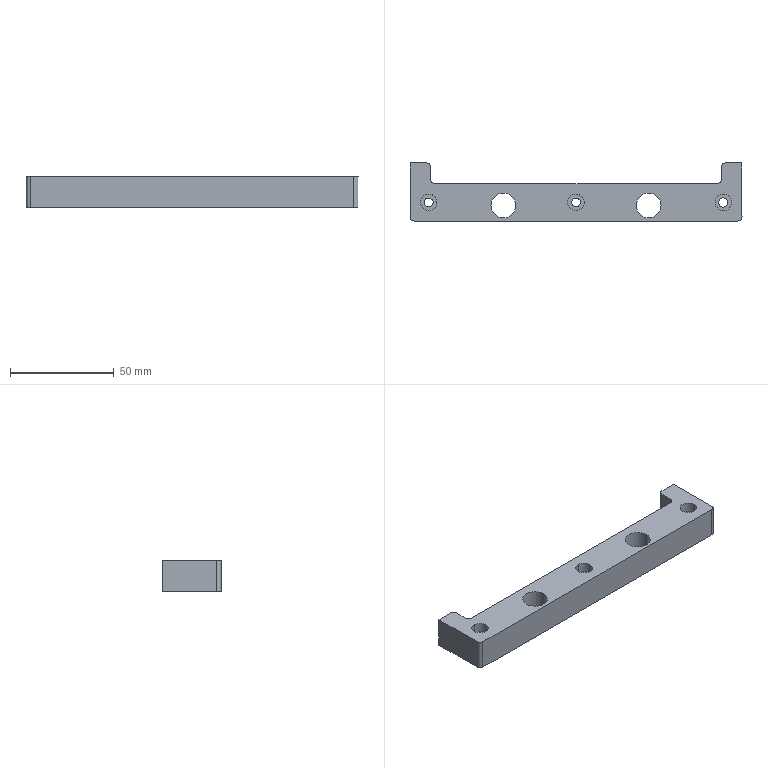Part | SolidWorks | features BaseBody 1, HoleWzd 1, MoveFace 1 | 1 solid | 39 faces | box 160 x 28 x 15 mm | volume 41591 mm3 | cylinder 26 | plane 13 | commonest cylinder face diameters 8 x8 4 x6 4.2 x6 12 x4 4.5 x2
STEP:
#1=CARTESIAN_POINT('',(-666.13,617.297,352.482));
#2=VERTEX_POINT('',#1);
#3=CARTESIAN_POINT('',(-658.13,617.297,352.482));
#4=VERTEX_POINT('',#3);
#5=CARTESIAN_POINT('',(-662.13,617.297,352.482));
#6=DIRECTION('',(0.,0.,1.));
#7=DIRECTION('',(1.,0.,0.));
#8=AXIS2_PLACEMENT_3D('',#5,#6,#7);
#9=CIRCLE('',#8,4.);
#10=EDGE_CURVE('',#2,#4,#9,.T.);
#11=ORIENTED_EDGE('',*,*,#10,.F.);
#12=CARTESIAN_POINT('',(-666.13,617.297,357.482));
#13=VERTEX_POINT('',#12);
#14=CARTESIAN_POINT('',(-666.13,617.297,357.482));
#15=DIRECTION('',(0.,0.,1.));
#16=VECTOR('',#15,1000.);
#17=LINE('',#14,#16);
#18=EDGE_CURVE('',#2,#13,#17,.T.);
#19=ORIENTED_EDGE('',*,*,#18,.T.);
#20=CARTESIAN_POINT('',(-658.13,617.297,357.482));
#21=VERTEX_POINT('',#20);
#22=CARTESIAN_POINT('',(-662.13,617.297,357.482));
#23=DIRECTION('',(0.,0.,1.));
#24=DIRECTION('',(1.,0.,0.));
#25=AXIS2_PLACEMENT_3D('',#22,#23,#24);
#26=CIRCLE('',#25,4.);
#27=EDGE_CURVE('',#13,#21,#26,.T.);
#28=ORIENTED_EDGE('',*,*,#27,.T.);
#29=CARTESIAN_POINT('',(-658.13,617.297,357.482));
#30=DIRECTION('',(0.,0.,1.));
#31=VECTOR('',#30,1000.);
#32=LINE('',#29,#31);
#33=EDGE_CURVE('',#4,#21,#32,.T.);
#34=ORIENTED_EDGE('',*,*,#33,.F.);
#35=EDGE_LOOP('',(#11,#19,#28,#34));
#36=FACE_OUTER_BOUND('',#35,.T.);
#37=CARTESIAN_POINT('',(-662.13,617.297,357.482));
#38=DIRECTION('',(0.,0.,1.));
#39=DIRECTION('',(1.,0.,0.));
#40=AXIS2_PLACEMENT_3D('',#37,#38,#39);
#41=CYLINDRICAL_SURFACE('',#40,4.);
#42=ADVANCED_FACE('',(#36),#41,.F.);
#43=CARTESIAN_POINT('',(-664.38,617.297,342.482));
#44=VERTEX_POINT('',#43);
#45=CARTESIAN_POINT('',(-659.88,617.297,342.482));
#46=VERTEX_POINT('',#45);
#47=CARTESIAN_POINT('',(-662.13,617.297,342.482));
#48=DIRECTION('',(0.,0.,1.));
#49=DIRECTION('',(1.,0.,0.));
#50=AXIS2_PLACEMENT_3D('',#47,#48,#49);
#51=CIRCLE('',#50,2.25);
#52=EDGE_CURVE('',#44,#46,#51,.T.);
#53=ORIENTED_EDGE('',*,*,#52,.F.);
#54=CARTESIAN_POINT('',(-664.38,617.297,352.482));
#55=VERTEX_POINT('',#54);
#56=CARTESIAN_POINT('',(-664.38,617.297,357.482));
#57=DIRECTION('',(0.,0.,1.));
#58=VECTOR('',#57,1000.);
#59=LINE('',#56,#58);
#60=EDGE_CURVE('',#44,#55,#59,.T.);
#61=ORIENTED_EDGE('',*,*,#60,.T.);
#62=CARTESIAN_POINT('',(-659.88,617.297,352.482));
#63=VERTEX_POINT('',#62);
#64=CARTESIAN_POINT('',(-662.13,617.297,352.482));
#65=DIRECTION('',(0.,0.,1.));
#66=DIRECTION('',(1.,0.,0.));
#67=AXIS2_PLACEMENT_3D('',#64,#65,#66);
#68=CIRCLE('',#67,2.25);
#69=EDGE_CURVE('',#55,#63,#68,.T.);
#70=ORIENTED_EDGE('',*,*,#69,.T.);
#71=CARTESIAN_POINT('',(-659.88,617.297,357.482));
#72=DIRECTION('',(0.,0.,1.));
#73=VECTOR('',#72,1000.);
#74=LINE('',#71,#73);
#75=EDGE_CURVE('',#46,#63,#74,.T.);
#76=ORIENTED_EDGE('',*,*,#75,.F.);
#77=EDGE_LOOP('',(#53,#61,#70,#76));
#78=FACE_OUTER_BOUND('',#77,.T.);
#79=CARTESIAN_POINT('',(-662.13,617.297,357.482));
#80=DIRECTION('',(0.,0.,1.));
#81=DIRECTION('',(1.,0.,0.));
#82=AXIS2_PLACEMENT_3D('',#79,#80,#81);
#83=CYLINDRICAL_SURFACE('',#82,2.25);
#84=ADVANCED_FACE('',(#78),#83,.F.);
#85=CARTESIAN_POINT('',(-733.13,615.197,342.482));
#86=VERTEX_POINT('',#85);
#87=CARTESIAN_POINT('',(-735.23,617.297,342.482));
#88=VERTEX_POINT('',#87);
#89=CARTESIAN_POINT('',(-733.13,617.297,342.482));
#90=DIRECTION('',(0.,0.,-1.));
#91=DIRECTION('',(-1.,-0.000001544,0.));
#92=AXIS2_PLACEMENT_3D('',#89,#90,#91);
#93=CIRCLE('',#92,2.1);
#94=EDGE_CURVE('',#86,#88,#93,.T.);
#95=ORIENTED_EDGE('',*,*,#94,.T.);
#96=CARTESIAN_POINT('',(-735.23,617.297,352.482));
#97=VERTEX_POINT('',#96);
#98=CARTESIAN_POINT('',(-735.23,617.297,357.482));
#99=DIRECTION('',(0.,0.,1.));
#100=VECTOR('',#99,1000.);
#101=LINE('',#98,#100);
#102=EDGE_CURVE('',#88,#97,#101,.T.);
#103=ORIENTED_EDGE('',*,*,#102,.T.);
#104=CARTESIAN_POINT('',(-733.13,615.197,352.482));
#105=VERTEX_POINT('',#104);
#106=CARTESIAN_POINT('',(-733.13,617.297,352.482));
#107=DIRECTION('',(0.,0.,1.));
#108=DIRECTION('',(-1.,-0.000001544,0.));
#109=AXIS2_PLACEMENT_3D('',#106,#107,#108);
#110=CIRCLE('',#109,2.1);
#111=EDGE_CURVE('',#97,#105,#110,.T.);
#112=ORIENTED_EDGE('',*,*,#111,.T.);
#113=CARTESIAN_POINT('',(-733.13,615.197,352.482));
#114=DIRECTION('',(0.,0.,-1.));
#115=VECTOR('',#114,1000.);
#116=LINE('',#113,#115);
#117=EDGE_CURVE('',#105,#86,#116,.T.);
#118=ORIENTED_EDGE('',*,*,#117,.T.);
#119=EDGE_LOOP('',(#95,#103,#112,#118));
#120=FACE_OUTER_BOUND('',#119,.T.);
#121=CARTESIAN_POINT('',(-733.13,617.297,357.482));
#122=DIRECTION('',(0.,0.,1.));
#123=DIRECTION('',(-1.,-0.000001544,0.));
#124=AXIS2_PLACEMENT_3D('',#121,#122,#123);
#125=CYLINDRICAL_SURFACE('',#124,2.1);
#126=ADVANCED_FACE('',(#120),#125,.F.);
#127=CARTESIAN_POINT('',(-733.13,613.297,352.482));
#128=VERTEX_POINT('',#127);
#129=CARTESIAN_POINT('',(-737.13,617.297,352.482));
#130=VERTEX_POINT('',#129);
#131=CARTESIAN_POINT('',(-733.13,617.297,352.482));
#132=DIRECTION('',(0.,0.,-1.));
#133=DIRECTION('',(-1.,-0.000001544,0.));
#134=AXIS2_PLACEMENT_3D('',#131,#132,#133);
#135=CIRCLE('',#134,4.);
#136=EDGE_CURVE('',#128,#130,#135,.T.);
#137=ORIENTED_EDGE('',*,*,#136,.T.);
#138=CARTESIAN_POINT('',(-737.13,617.297,357.482));
#139=VERTEX_POINT('',#138);
#140=CARTESIAN_POINT('',(-737.13,617.297,357.482));
#141=DIRECTION('',(0.,0.,1.));
#142=VECTOR('',#141,1000.);
#143=LINE('',#140,#142);
#144=EDGE_CURVE('',#130,#139,#143,.T.);
#145=ORIENTED_EDGE('',*,*,#144,.T.);
#146=CARTESIAN_POINT('',(-733.13,613.297,357.482));
#147=VERTEX_POINT('',#146);
#148=CARTESIAN_POINT('',(-733.13,617.297,357.482));
#149=DIRECTION('',(0.,0.,1.));
#150=DIRECTION('',(-1.,-0.000001544,0.));
#151=AXIS2_PLACEMENT_3D('',#148,#149,#150);
#152=CIRCLE('',#151,4.);
#153=EDGE_CURVE('',#139,#147,#152,.T.);
#154=ORIENTED_EDGE('',*,*,#153,.T.);
#155=CARTESIAN_POINT('',(-733.13,613.297,357.482));
#156=DIRECTION('',(0.,0.,-1.));
#157=VECTOR('',#156,1000.);
#158=LINE('',#155,#157);
#159=EDGE_CURVE('',#147,#128,#158,.T.);
#160=ORIENTED_EDGE('',*,*,#159,.T.);
#161=EDGE_LOOP('',(#137,#145,#154,#160));
#162=FACE_OUTER_BOUND('',#161,.T.);
#163=CARTESIAN_POINT('',(-733.13,617.297,357.482));
#164=DIRECTION('',(0.,0.,1.));
#165=DIRECTION('',(-1.,-0.000001544,0.));
#166=AXIS2_PLACEMENT_3D('',#163,#164,#165);
#167=CYLINDRICAL_SURFACE('',#166,4.);
#168=ADVANCED_FACE('',(#162),#167,.F.);
#169=CARTESIAN_POINT('',(-804.13,615.197,342.482));
#170=VERTEX_POINT('',#169);
#171=CARTESIAN_POINT('',(-806.23,617.297,342.482));
#172=VERTEX_POINT('',#171);
#173=CARTESIAN_POINT('',(-804.13,617.297,342.482));
#174=DIRECTION('',(0.,0.,-1.));
#175=DIRECTION('',(-1.,-0.000001544,0.));
#176=AXIS2_PLACEMENT_3D('',#173,#174,#175);
#177=CIRCLE('',#176,2.1);
#178=EDGE_CURVE('',#170,#172,#177,.T.);
#179=ORIENTED_EDGE('',*,*,#178,.T.);
#180=CARTESIAN_POINT('',(-806.23,617.297,352.482));
#181=VERTEX_POINT('',#180);
#182=CARTESIAN_POINT('',(-806.23,617.297,357.482));
#183=DIRECTION('',(0.,0.,1.));
#184=VECTOR('',#183,1000.);
#185=LINE('',#182,#184);
#186=EDGE_CURVE('',#172,#181,#185,.T.);
#187=ORIENTED_EDGE('',*,*,#186,.T.);
#188=CARTESIAN_POINT('',(-804.13,615.197,352.482));
#189=VERTEX_POINT('',#188);
#190=CARTESIAN_POINT('',(-804.13,617.297,352.482));
#191=DIRECTION('',(0.,0.,1.));
#192=DIRECTION('',(-1.,-0.000001544,0.));
#193=AXIS2_PLACEMENT_3D('',#190,#191,#192);
#194=CIRCLE('',#193,2.1);
#195=EDGE_CURVE('',#181,#189,#194,.T.);
#196=ORIENTED_EDGE('',*,*,#195,.T.);
#197=CARTESIAN_POINT('',(-804.13,615.197,352.482));
#198=DIRECTION('',(0.,0.,-1.));
#199=VECTOR('',#198,1000.);
#200=LINE('',#197,#199);
#201=EDGE_CURVE('',#189,#170,#200,.T.);
#202=ORIENTED_EDGE('',*,*,#201,.T.);
#203=EDGE_LOOP('',(#179,#187,#196,#202));
#204=FACE_OUTER_BOUND('',#203,.T.);
#205=CARTESIAN_POINT('',(-804.13,617.297,357.482));
#206=DIRECTION('',(0.,0.,1.));
#207=DIRECTION('',(-1.,-0.000001544,0.));
#208=AXIS2_PLACEMENT_3D('',#205,#206,#207);
#209=CYLINDRICAL_SURFACE('',#208,2.1);
#210=ADVANCED_FACE('',(#204),#209,.F.);
#211=CARTESIAN_POINT('',(-804.13,613.297,352.482));
#212=VERTEX_POINT('',#211);
#213=CARTESIAN_POINT('',(-808.13,617.297,352.482));
#214=VERTEX_POINT('',#213);
#215=CARTESIAN_POINT('',(-804.13,617.297,352.482));
#216=DIRECTION('',(0.,0.,-1.));
#217=DIRECTION('',(-1.,-0.000001544,0.));
#218=AXIS2_PLACEMENT_3D('',#215,#216,#217);
#219=CIRCLE('',#218,4.);
#220=EDGE_CURVE('',#212,#214,#219,.T.);
#221=ORIENTED_EDGE('',*,*,#220,.T.);
#222=CARTESIAN_POINT('',(-808.13,617.297,357.482));
#223=VERTEX_POINT('',#222);
#224=CARTESIAN_POINT('',(-808.13,617.297,357.482));
#225=DIRECTION('',(0.,0.,1.));
#226=VECTOR('',#225,1000.);
#227=LINE('',#224,#226);
#228=EDGE_CURVE('',#214,#223,#227,.T.);
#229=ORIENTED_EDGE('',*,*,#228,.T.);
#230=CARTESIAN_POINT('',(-804.13,613.297,357.482));
#231=VERTEX_POINT('',#230);
#232=CARTESIAN_POINT('',(-804.13,617.297,357.482));
#233=DIRECTION('',(0.,0.,1.));
#234=DIRECTION('',(-1.,-0.000001544,0.));
#235=AXIS2_PLACEMENT_3D('',#232,#233,#234);
#236=CIRCLE('',#235,4.);
#237=EDGE_CURVE('',#223,#231,#236,.T.);
#238=ORIENTED_EDGE('',*,*,#237,.T.);
#239=CARTESIAN_POINT('',(-804.13,613.297,357.482));
#240=DIRECTION('',(0.,0.,-1.));
#241=VECTOR('',#240,1000.);
#242=LINE('',#239,#241);
#243=EDGE_CURVE('',#231,#212,#242,.T.);
#244=ORIENTED_EDGE('',*,*,#243,.T.);
#245=EDGE_LOOP('',(#221,#229,#238,#244));
#246=FACE_OUTER_BOUND('',#245,.T.);
#247=CARTESIAN_POINT('',(-804.13,617.297,357.482));
#248=DIRECTION('',(0.,0.,1.));
#249=DIRECTION('',(-1.,-0.000001544,0.));
#250=AXIS2_PLACEMENT_3D('',#247,#248,#249);
#251=CYLINDRICAL_SURFACE('',#250,4.);
#252=ADVANCED_FACE('',(#246),#251,.F.);
#253=CARTESIAN_POINT('',(-774.13,615.797,342.482));
#254=VERTEX_POINT('',#253);
#255=CARTESIAN_POINT('',(-762.13,615.797,342.482));
#256=VERTEX_POINT('',#255);
#257=CARTESIAN_POINT('',(-768.13,615.797,342.482));
#258=DIRECTION('',(0.,0.,-1.));
#259=DIRECTION('',(-1.,-0.000001544,0.));
#260=AXIS2_PLACEMENT_3D('',#257,#258,#259);
#261=CIRCLE('',#260,6.);
#262=EDGE_CURVE('',#254,#256,#261,.T.);
#263=ORIENTED_EDGE('',*,*,#262,.F.);
#264=CARTESIAN_POINT('',(-768.13,615.797,342.482));
#265=DIRECTION('',(0.,0.,-1.));
#266=DIRECTION('',(1.,0.000001544,0.));
#267=AXIS2_PLACEMENT_3D('',#264,#265,#266);
#268=CIRCLE('',#267,6.);
#269=EDGE_CURVE('',#256,#254,#268,.T.);
#270=ORIENTED_EDGE('',*,*,#269,.F.);
#271=EDGE_LOOP('',(#263,#270));
#272=FACE_BOUND('',#271,.T.);
#273=CARTESIAN_POINT('',(-704.13,615.797,342.482));
#274=VERTEX_POINT('',#273);
#275=CARTESIAN_POINT('',(-692.13,615.797,342.482));
#276=VERTEX_POINT('',#275);
#277=CARTESIAN_POINT('',(-698.13,615.797,342.482));
#278=DIRECTION('',(0.,0.,-1.));
#279=DIRECTION('',(-1.,-0.000001544,0.));
#280=AXIS2_PLACEMENT_3D('',#277,#278,#279);
#281=CIRCLE('',#280,6.);
#282=EDGE_CURVE('',#274,#276,#281,.T.);
#283=ORIENTED_EDGE('',*,*,#282,.F.);
#284=CARTESIAN_POINT('',(-698.13,615.797,342.482));
#285=DIRECTION('',(0.,0.,-1.));
#286=DIRECTION('',(1.,0.000001544,0.));
#287=AXIS2_PLACEMENT_3D('',#284,#285,#286);
#288=CIRCLE('',#287,6.);
#289=EDGE_CURVE('',#276,#274,#288,.T.);
#290=ORIENTED_EDGE('',*,*,#289,.F.);
#291=EDGE_LOOP('',(#283,#290));
#292=FACE_BOUND('',#291,.T.);
#293=ORIENTED_EDGE('',*,*,#94,.F.);
#294=CARTESIAN_POINT('',(-733.13,619.397,342.482));
#295=VERTEX_POINT('',#294);
#296=CARTESIAN_POINT('',(-733.13,617.297,342.482));
#297=DIRECTION('',(0.,0.,-1.));
#298=DIRECTION('',(-0.000001544,1.,0.));
#299=AXIS2_PLACEMENT_3D('',#296,#297,#298);
#300=CIRCLE('',#299,2.1);
#301=EDGE_CURVE('',#295,#86,#300,.T.);
#302=ORIENTED_EDGE('',*,*,#301,.F.);
#303=CARTESIAN_POINT('',(-733.13,617.297,342.482));
#304=DIRECTION('',(0.,0.,-1.));
#305=DIRECTION('',(-1.,-0.000001544,0.));
#306=AXIS2_PLACEMENT_3D('',#303,#304,#305);
#307=CIRCLE('',#306,2.1);
#308=EDGE_CURVE('',#88,#295,#307,.T.);
#309=ORIENTED_EDGE('',*,*,#308,.F.);
#310=EDGE_LOOP('',(#293,#302,#309));
#311=FACE_BOUND('',#310,.T.);
#312=ORIENTED_EDGE('',*,*,#178,.F.);
#313=CARTESIAN_POINT('',(-804.13,619.397,342.482));
#314=VERTEX_POINT('',#313);
#315=CARTESIAN_POINT('',(-804.13,617.297,342.482));
#316=DIRECTION('',(0.,0.,-1.));
#317=DIRECTION('',(-0.000001544,1.,0.));
#318=AXIS2_PLACEMENT_3D('',#315,#316,#317);
#319=CIRCLE('',#318,2.1);
#320=EDGE_CURVE('',#314,#170,#319,.T.);
#321=ORIENTED_EDGE('',*,*,#320,.F.);
#322=CARTESIAN_POINT('',(-804.13,617.297,342.482));
#323=DIRECTION('',(0.,0.,-1.));
#324=DIRECTION('',(-1.,-0.000001544,0.));
#325=AXIS2_PLACEMENT_3D('',#322,#323,#324);
#326=CIRCLE('',#325,2.1);
#327=EDGE_CURVE('',#172,#314,#326,.T.);
#328=ORIENTED_EDGE('',*,*,#327,.F.);
#329=EDGE_LOOP('',(#312,#321,#328));
#330=FACE_BOUND('',#329,.T.);
#331=CARTESIAN_POINT('',(-653.13,636.297,342.482));
#332=VERTEX_POINT('',#331);
#333=CARTESIAN_POINT('',(-661.13,636.297,342.482));
#334=VERTEX_POINT('',#333);
#335=CARTESIAN_POINT('',(-653.13,636.297,342.482));
#336=DIRECTION('',(-1.,-0.000001544,0.));
#337=VECTOR('',#336,1000.);
#338=LINE('',#335,#337);
#339=EDGE_CURVE('',#332,#334,#338,.T.);
#340=ORIENTED_EDGE('',*,*,#339,.F.);
#341=CARTESIAN_POINT('',(-653.13,610.297,342.482));
#342=VERTEX_POINT('',#341);
#343=CARTESIAN_POINT('',(-653.13,610.297,342.482));
#344=DIRECTION('',(-0.000001544,1.,0.));
#345=VECTOR('',#344,1000.);
#346=LINE('',#343,#345);
#347=EDGE_CURVE('',#342,#332,#346,.T.);
#348=ORIENTED_EDGE('',*,*,#347,.F.);
#349=CARTESIAN_POINT('',(-655.13,608.297,342.482));
#350=VERTEX_POINT('',#349);
#351=CARTESIAN_POINT('',(-655.13,610.297,342.482));
#352=DIRECTION('',(0.,0.,1.));
#353=DIRECTION('',(0.000001545,-1.,0.));
#354=AXIS2_PLACEMENT_3D('',#351,#352,#353);
#355=CIRCLE('',#354,2.);
#356=EDGE_CURVE('',#350,#342,#355,.T.);
#357=ORIENTED_EDGE('',*,*,#356,.F.);
#358=CARTESIAN_POINT('',(-811.13,608.297,342.482));
#359=VERTEX_POINT('',#358);
#360=CARTESIAN_POINT('',(-811.13,608.297,342.482));
#361=DIRECTION('',(1.,0.000001544,0.));
#362=VECTOR('',#361,1000.);
#363=LINE('',#360,#362);
#364=EDGE_CURVE('',#359,#350,#363,.T.);
#365=ORIENTED_EDGE('',*,*,#364,.F.);
#366=CARTESIAN_POINT('',(-813.13,610.297,342.482));
#367=VERTEX_POINT('',#366);
#368=CARTESIAN_POINT('',(-811.13,610.297,342.482));
#369=DIRECTION('',(0.,0.,1.));
#370=DIRECTION('',(-1.,-0.000001545,0.));
#371=AXIS2_PLACEMENT_3D('',#368,#369,#370);
#372=CIRCLE('',#371,2.);
#373=EDGE_CURVE('',#367,#359,#372,.T.);
#374=ORIENTED_EDGE('',*,*,#373,.F.);
#375=CARTESIAN_POINT('',(-813.13,636.297,342.482));
#376=VERTEX_POINT('',#375);
#377=CARTESIAN_POINT('',(-813.13,636.297,342.482));
#378=DIRECTION('',(0.000001544,-1.,0.));
#379=VECTOR('',#378,1000.);
#380=LINE('',#377,#379);
#381=EDGE_CURVE('',#376,#367,#380,.T.);
#382=ORIENTED_EDGE('',*,*,#381,.F.);
#383=CARTESIAN_POINT('',(-805.13,636.297,342.482));
#384=VERTEX_POINT('',#383);
#385=CARTESIAN_POINT('',(-805.13,636.297,342.482));
#386=DIRECTION('',(-1.,-0.000001544,0.));
#387=VECTOR('',#386,1000.);
#388=LINE('',#385,#387);
#389=EDGE_CURVE('',#384,#376,#388,.T.);
#390=ORIENTED_EDGE('',*,*,#389,.F.);
#391=CARTESIAN_POINT('',(-803.13,634.297,342.482));
#392=VERTEX_POINT('',#391);
#393=CARTESIAN_POINT('',(-805.13,634.297,342.482));
#394=DIRECTION('',(0.,0.,1.));
#395=DIRECTION('',(1.,0.000001543,0.));
#396=AXIS2_PLACEMENT_3D('',#393,#394,#395);
#397=CIRCLE('',#396,2.);
#398=EDGE_CURVE('',#392,#384,#397,.T.);
#399=ORIENTED_EDGE('',*,*,#398,.F.);
#400=CARTESIAN_POINT('',(-803.13,628.297,342.482));
#401=VERTEX_POINT('',#400);
#402=CARTESIAN_POINT('',(-803.13,634.297,342.482));
#403=DIRECTION('',(0.000001544,-1.,0.));
#404=VECTOR('',#403,1000.);
#405=LINE('',#402,#404);
#406=EDGE_CURVE('',#392,#401,#405,.T.);
#407=ORIENTED_EDGE('',*,*,#406,.T.);
#408=CARTESIAN_POINT('',(-801.13,626.297,342.482));
#409=VERTEX_POINT('',#408);
#410=CARTESIAN_POINT('',(-801.13,628.297,342.482));
#411=DIRECTION('',(0.,0.,-1.));
#412=DIRECTION('',(0.000001545,-1.,0.));
#413=AXIS2_PLACEMENT_3D('',#410,#411,#412);
#414=CIRCLE('',#413,2.);
#415=EDGE_CURVE('',#409,#401,#414,.T.);
#416=ORIENTED_EDGE('',*,*,#415,.F.);
#417=CARTESIAN_POINT('',(-665.13,626.297,342.482));
#418=VERTEX_POINT('',#417);
#419=CARTESIAN_POINT('',(-801.13,626.297,342.482));
#420=DIRECTION('',(1.,0.000001544,0.));
#421=VECTOR('',#420,1000.);
#422=LINE('',#419,#421);
#423=EDGE_CURVE('',#409,#418,#422,.T.);
#424=ORIENTED_EDGE('',*,*,#423,.T.);
#425=CARTESIAN_POINT('',(-663.13,628.297,342.482));
#426=VERTEX_POINT('',#425);
#427=CARTESIAN_POINT('',(-665.13,628.297,342.482));
#428=DIRECTION('',(0.,0.,-1.));
#429=DIRECTION('',(1.,0.000001545,0.));
#430=AXIS2_PLACEMENT_3D('',#427,#428,#429);
#431=CIRCLE('',#430,2.);
#432=EDGE_CURVE('',#426,#418,#431,.T.);
#433=ORIENTED_EDGE('',*,*,#432,.F.);
#434=CARTESIAN_POINT('',(-663.13,634.297,342.482));
#435=VERTEX_POINT('',#434);
#436=CARTESIAN_POINT('',(-663.13,634.297,342.482));
#437=DIRECTION('',(0.000001544,-1.,0.));
#438=VECTOR('',#437,1000.);
#439=LINE('',#436,#438);
#440=EDGE_CURVE('',#435,#426,#439,.T.);
#441=ORIENTED_EDGE('',*,*,#440,.F.);
#442=CARTESIAN_POINT('',(-661.13,634.297,342.482));
#443=DIRECTION('',(0.,0.,1.));
#444=DIRECTION('',(-0.000001544,1.,0.));
#445=AXIS2_PLACEMENT_3D('',#442,#443,#444);
#446=CIRCLE('',#445,2.);
#447=EDGE_CURVE('',#334,#435,#446,.T.);
#448=ORIENTED_EDGE('',*,*,#447,.F.);
#449=EDGE_LOOP('',(#340,#348,#357,#365,#374,#382,#390,#399,#407,#416,#424,#433,#441,#448));
#450=FACE_OUTER_BOUND('',#449,.T.);
#451=CARTESIAN_POINT('',(-662.13,617.297,342.482));
#452=DIRECTION('',(0.,0.,1.));
#453=DIRECTION('',(1.,0.,0.));
#454=AXIS2_PLACEMENT_3D('',#451,#452,#453);
#455=CIRCLE('',#454,2.25);
#456=EDGE_CURVE('',#46,#44,#455,.T.);
#457=ORIENTED_EDGE('',*,*,#456,.T.);
#458=ORIENTED_EDGE('',*,*,#52,.T.);
#459=EDGE_LOOP('',(#457,#458));
#460=FACE_BOUND('',#459,.T.);
#461=CARTESIAN_POINT('',(-653.13,608.297,342.482));
#462=DIRECTION('',(0.,0.,-1.));
#463=DIRECTION('',(0.000001544,-1.,0.));
#464=AXIS2_PLACEMENT_3D('',#461,#462,#463);
#465=PLANE('',#464);
#466=ADVANCED_FACE('',(#272,#292,#311,#330,#450,#460),#465,.T.);
#467=CARTESIAN_POINT('',(-803.13,634.297,357.482));
#468=VERTEX_POINT('',#467);
#469=CARTESIAN_POINT('',(-803.13,634.297,342.482));
#470=DIRECTION('',(0.,0.,1.));
#471=VECTOR('',#470,1000.);
#472=LINE('',#469,#471);
#473=EDGE_CURVE('',#392,#468,#472,.T.);
#474=ORIENTED_EDGE('',*,*,#473,.T.);
#475=CARTESIAN_POINT('',(-803.13,628.297,357.482));
#476=VERTEX_POINT('',#475);
#477=CARTESIAN_POINT('',(-803.13,628.297,357.482));
#478=DIRECTION('',(-0.000001544,1.,0.));
#479=VECTOR('',#478,1000.);
#480=LINE('',#477,#479);
#481=EDGE_CURVE('',#476,#468,#480,.T.);
#482=ORIENTED_EDGE('',*,*,#481,.F.);
#483=CARTESIAN_POINT('',(-803.13,628.297,357.482));
#484=DIRECTION('',(0.,0.,-1.));
#485=VECTOR('',#484,1000.);
#486=LINE('',#483,#485);
#487=EDGE_CURVE('',#476,#401,#486,.T.);
#488=ORIENTED_EDGE('',*,*,#487,.T.);
#489=ORIENTED_EDGE('',*,*,#406,.F.);
#490=EDGE_LOOP('',(#474,#482,#488,#489));
#491=FACE_OUTER_BOUND('',#490,.T.);
#492=CARTESIAN_POINT('',(-803.13,626.297,357.482));
#493=DIRECTION('',(1.,0.000001544,0.));
#494=DIRECTION('',(0.000001544,-1.,0.));
#495=AXIS2_PLACEMENT_3D('',#492,#493,#494);
#496=PLANE('',#495);
#497=ADVANCED_FACE('',(#491),#496,.T.);
#498=CARTESIAN_POINT('',(-663.13,634.297,357.482));
#499=VERTEX_POINT('',#498);
#500=CARTESIAN_POINT('',(-661.13,636.297,357.482));
#501=VERTEX_POINT('',#500);
#502=CARTESIAN_POINT('',(-661.13,634.297,357.482));
#503=DIRECTION('',(0.,0.,-1.));
#504=DIRECTION('',(-1.,-0.000001544,0.));
#505=AXIS2_PLACEMENT_3D('',#502,#503,#504);
#506=CIRCLE('',#505,2.);
#507=EDGE_CURVE('',#499,#501,#506,.T.);
#508=ORIENTED_EDGE('',*,*,#507,.T.);
#509=CARTESIAN_POINT('',(-661.13,636.297,342.482));
#510=DIRECTION('',(0.,0.,1.));
#511=VECTOR('',#510,1000.);
#512=LINE('',#509,#511);
#513=EDGE_CURVE('',#334,#501,#512,.T.);
#514=ORIENTED_EDGE('',*,*,#513,.F.);
#515=ORIENTED_EDGE('',*,*,#447,.T.);
#516=CARTESIAN_POINT('',(-663.13,634.297,357.482));
#517=DIRECTION('',(0.,0.,-1.));
#518=VECTOR('',#517,1000.);
#519=LINE('',#516,#518);
#520=EDGE_CURVE('',#499,#435,#519,.T.);
#521=ORIENTED_EDGE('',*,*,#520,.F.);
#522=EDGE_LOOP('',(#508,#514,#515,#521));
#523=FACE_OUTER_BOUND('',#522,.T.);
#524=CARTESIAN_POINT('',(-661.13,634.297,494.293));
#525=DIRECTION('',(0.,0.,-1.));
#526=DIRECTION('',(1.,0.000001544,0.));
#527=AXIS2_PLACEMENT_3D('',#524,#525,#526);
#528=CYLINDRICAL_SURFACE('',#527,2.);
#529=ADVANCED_FACE('',(#523),#528,.T.);
#530=ORIENTED_EDGE('',*,*,#520,.T.);
#531=ORIENTED_EDGE('',*,*,#440,.T.);
#532=CARTESIAN_POINT('',(-663.13,628.297,357.482));
#533=VERTEX_POINT('',#532);
#534=CARTESIAN_POINT('',(-663.13,628.297,342.482));
#535=DIRECTION('',(0.,0.,1.));
#536=VECTOR('',#535,1000.);
#537=LINE('',#534,#536);
#538=EDGE_CURVE('',#426,#533,#537,.T.);
#539=ORIENTED_EDGE('',*,*,#538,.T.);
#540=CARTESIAN_POINT('',(-663.13,634.297,357.482));
#541=DIRECTION('',(0.000001544,-1.,0.));
#542=VECTOR('',#541,1000.);
#543=LINE('',#540,#542);
#544=EDGE_CURVE('',#499,#533,#543,.T.);
#545=ORIENTED_EDGE('',*,*,#544,.F.);
#546=EDGE_LOOP('',(#530,#531,#539,#545));
#547=FACE_OUTER_BOUND('',#546,.T.);
#548=CARTESIAN_POINT('',(-663.13,636.297,357.482));
#549=DIRECTION('',(-1.,-0.000001544,0.));
#550=DIRECTION('',(-0.000001544,1.,0.));
#551=AXIS2_PLACEMENT_3D('',#548,#549,#550);
#552=PLANE('',#551);
#553=ADVANCED_FACE('',(#547),#552,.T.);
#554=CARTESIAN_POINT('',(-662.13,617.297,357.482));
#555=DIRECTION('',(0.,0.,1.));
#556=DIRECTION('',(1.,0.,0.));
#557=AXIS2_PLACEMENT_3D('',#554,#555,#556);
#558=CIRCLE('',#557,4.);
#559=EDGE_CURVE('',#21,#13,#558,.T.);
#560=ORIENTED_EDGE('',*,*,#559,.F.);
#561=ORIENTED_EDGE('',*,*,#27,.F.);
#562=EDGE_LOOP('',(#560,#561));
#563=FACE_BOUND('',#562,.T.);
#564=ORIENTED_EDGE('',*,*,#481,.T.);
#565=CARTESIAN_POINT('',(-805.13,636.297,357.482));
#566=VERTEX_POINT('',#565);
#567=CARTESIAN_POINT('',(-805.13,634.297,357.482));
#568=DIRECTION('',(0.,0.,-1.));
#569=DIRECTION('',(-0.000001544,1.,0.));
#570=AXIS2_PLACEMENT_3D('',#567,#568,#569);
#571=CIRCLE('',#570,2.);
#572=EDGE_CURVE('',#566,#468,#571,.T.);
#573=ORIENTED_EDGE('',*,*,#572,.F.);
#574=CARTESIAN_POINT('',(-813.13,636.297,357.482));
#575=VERTEX_POINT('',#574);
#576=CARTESIAN_POINT('',(-813.13,636.297,357.482));
#577=DIRECTION('',(1.,0.000001544,0.));
#578=VECTOR('',#577,1000.);
#579=LINE('',#576,#578);
#580=EDGE_CURVE('',#575,#566,#579,.T.);
#581=ORIENTED_EDGE('',*,*,#580,.F.);
#582=CARTESIAN_POINT('',(-813.13,610.297,357.482));
#583=VERTEX_POINT('',#582);
#584=CARTESIAN_POINT('',(-813.13,610.297,357.482));
#585=DIRECTION('',(-0.000001544,1.,0.));
#586=VECTOR('',#585,1000.);
#587=LINE('',#584,#586);
#588=EDGE_CURVE('',#583,#575,#587,.T.);
#589=ORIENTED_EDGE('',*,*,#588,.F.);
#590=CARTESIAN_POINT('',(-811.13,608.297,357.482));
#591=VERTEX_POINT('',#590);
#592=CARTESIAN_POINT('',(-811.13,610.297,357.482));
#593=DIRECTION('',(0.,0.,-1.));
#594=DIRECTION('',(0.000001545,-1.,0.));
#595=AXIS2_PLACEMENT_3D('',#592,#593,#594);
#596=CIRCLE('',#595,2.);
#597=EDGE_CURVE('',#591,#583,#596,.T.);
#598=ORIENTED_EDGE('',*,*,#597,.F.);
#599=CARTESIAN_POINT('',(-655.13,608.297,357.482));
#600=VERTEX_POINT('',#599);
#601=CARTESIAN_POINT('',(-655.13,608.297,357.482));
#602=DIRECTION('',(-1.,-0.000001544,0.));
#603=VECTOR('',#602,1000.);
#604=LINE('',#601,#603);
#605=EDGE_CURVE('',#600,#591,#604,.T.);
#606=ORIENTED_EDGE('',*,*,#605,.F.);
#607=CARTESIAN_POINT('',(-653.13,610.297,357.482));
#608=VERTEX_POINT('',#607);
#609=CARTESIAN_POINT('',(-655.13,610.297,357.482));
#610=DIRECTION('',(0.,0.,-1.));
#611=DIRECTION('',(1.,0.000001544,0.));
#612=AXIS2_PLACEMENT_3D('',#609,#610,#611);
#613=CIRCLE('',#612,2.);
#614=EDGE_CURVE('',#608,#600,#613,.T.);
#615=ORIENTED_EDGE('',*,*,#614,.F.);
#616=CARTESIAN_POINT('',(-653.13,636.297,357.482));
#617=VERTEX_POINT('',#616);
#618=CARTESIAN_POINT('',(-653.13,636.297,357.482));
#619=DIRECTION('',(0.000001544,-1.,0.));
#620=VECTOR('',#619,1000.);
#621=LINE('',#618,#620);
#622=EDGE_CURVE('',#617,#608,#621,.T.);
#623=ORIENTED_EDGE('',*,*,#622,.F.);
#624=CARTESIAN_POINT('',(-661.13,636.297,357.482));
#625=DIRECTION('',(1.,0.000001544,0.));
#626=VECTOR('',#625,1000.);
#627=LINE('',#624,#626);
#628=EDGE_CURVE('',#501,#617,#627,.T.);
#629=ORIENTED_EDGE('',*,*,#628,.F.);
#630=ORIENTED_EDGE('',*,*,#507,.F.);
#631=ORIENTED_EDGE('',*,*,#544,.T.);
#632=CARTESIAN_POINT('',(-665.13,626.297,357.482));
#633=VERTEX_POINT('',#632);
#634=CARTESIAN_POINT('',(-665.13,628.297,357.482));
#635=DIRECTION('',(0.,0.,1.));
#636=DIRECTION('',(0.000001545,-1.,0.));
#637=AXIS2_PLACEMENT_3D('',#634,#635,#636);
#638=CIRCLE('',#637,2.);
#639=EDGE_CURVE('',#633,#533,#638,.T.);
#640=ORIENTED_EDGE('',*,*,#639,.F.);
#641=CARTESIAN_POINT('',(-801.13,626.297,357.482));
#642=VERTEX_POINT('',#641);
#643=CARTESIAN_POINT('',(-665.13,626.297,357.482));
#644=DIRECTION('',(-1.,-0.000001544,0.));
#645=VECTOR('',#644,1000.);
#646=LINE('',#643,#645);
#647=EDGE_CURVE('',#633,#642,#646,.T.);
#648=ORIENTED_EDGE('',*,*,#647,.T.);
#649=CARTESIAN_POINT('',(-801.13,628.297,357.482));
#650=DIRECTION('',(0.,0.,1.));
#651=DIRECTION('',(-1.,-0.000001544,0.));
#652=AXIS2_PLACEMENT_3D('',#649,#650,#651);
#653=CIRCLE('',#652,2.);
#654=EDGE_CURVE('',#476,#642,#653,.T.);
#655=ORIENTED_EDGE('',*,*,#654,.F.);
#656=EDGE_LOOP('',(#564,#573,#581,#589,#598,#606,#615,#623,#629,#630,#631,#640,#648,#655));
#657=FACE_OUTER_BOUND('',#656,.T.);
#658=CARTESIAN_POINT('',(-804.13,621.297,357.482));
#659=VERTEX_POINT('',#658);
#660=CARTESIAN_POINT('',(-804.13,617.297,357.482));
#661=DIRECTION('',(0.,0.,1.));
#662=DIRECTION('',(-1.,-0.000001544,0.));
#663=AXIS2_PLACEMENT_3D('',#660,#661,#662);
#664=CIRCLE('',#663,4.);
#665=EDGE_CURVE('',#659,#223,#664,.T.);
#666=ORIENTED_EDGE('',*,*,#665,.F.);
#667=CARTESIAN_POINT('',(-804.13,617.297,357.482));
#668=DIRECTION('',(0.,0.,1.));
#669=DIRECTION('',(0.000001544,-1.,0.));
#670=AXIS2_PLACEMENT_3D('',#667,#668,#669);
#671=CIRCLE('',#670,4.);
#672=EDGE_CURVE('',#231,#659,#671,.T.);
#673=ORIENTED_EDGE('',*,*,#672,.F.);
#674=ORIENTED_EDGE('',*,*,#237,.F.);
#675=EDGE_LOOP('',(#666,#673,#674));
#676=FACE_BOUND('',#675,.T.);
#677=CARTESIAN_POINT('',(-733.13,621.297,357.482));
#678=VERTEX_POINT('',#677);
#679=CARTESIAN_POINT('',(-733.13,617.297,357.482));
#680=DIRECTION('',(0.,0.,1.));
#681=DIRECTION('',(-1.,-0.000001544,0.));
#682=AXIS2_PLACEMENT_3D('',#679,#680,#681);
#683=CIRCLE('',#682,4.);
#684=EDGE_CURVE('',#678,#139,#683,.T.);
#685=ORIENTED_EDGE('',*,*,#684,.F.);
#686=CARTESIAN_POINT('',(-733.13,617.297,357.482));
#687=DIRECTION('',(0.,0.,1.));
#688=DIRECTION('',(0.000001544,-1.,0.));
#689=AXIS2_PLACEMENT_3D('',#686,#687,#688);
#690=CIRCLE('',#689,4.);
#691=EDGE_CURVE('',#147,#678,#690,.T.);
#692=ORIENTED_EDGE('',*,*,#691,.F.);
#693=ORIENTED_EDGE('',*,*,#153,.F.);
#694=EDGE_LOOP('',(#685,#692,#693));
#695=FACE_BOUND('',#694,.T.);
#696=CARTESIAN_POINT('',(-692.13,615.797,357.482));
#697=VERTEX_POINT('',#696);
#698=CARTESIAN_POINT('',(-704.13,615.797,357.482));
#699=VERTEX_POINT('',#698);
#700=CARTESIAN_POINT('',(-698.13,615.797,357.482));
#701=DIRECTION('',(0.,0.,1.));
#702=DIRECTION('',(1.,0.000001544,0.));
#703=AXIS2_PLACEMENT_3D('',#700,#701,#702);
#704=CIRCLE('',#703,6.);
#705=EDGE_CURVE('',#697,#699,#704,.T.);
#706=ORIENTED_EDGE('',*,*,#705,.F.);
#707=CARTESIAN_POINT('',(-698.13,615.797,357.482));
#708=DIRECTION('',(0.,0.,1.));
#709=DIRECTION('',(-1.,-0.000001544,0.));
#710=AXIS2_PLACEMENT_3D('',#707,#708,#709);
#711=CIRCLE('',#710,6.);
#712=EDGE_CURVE('',#699,#697,#711,.T.);
#713=ORIENTED_EDGE('',*,*,#712,.F.);
#714=EDGE_LOOP('',(#706,#713));
#715=FACE_BOUND('',#714,.T.);
#716=CARTESIAN_POINT('',(-762.13,615.797,357.482));
#717=VERTEX_POINT('',#716);
#718=CARTESIAN_POINT('',(-774.13,615.797,357.482));
#719=VERTEX_POINT('',#718);
#720=CARTESIAN_POINT('',(-768.13,615.797,357.482));
#721=DIRECTION('',(0.,0.,1.));
#722=DIRECTION('',(1.,0.000001544,0.));
#723=AXIS2_PLACEMENT_3D('',#720,#721,#722);
#724=CIRCLE('',#723,6.);
#725=EDGE_CURVE('',#717,#719,#724,.T.);
#726=ORIENTED_EDGE('',*,*,#725,.F.);
#727=CARTESIAN_POINT('',(-768.13,615.797,357.482));
#728=DIRECTION('',(0.,0.,1.));
#729=DIRECTION('',(-1.,-0.000001544,0.));
#730=AXIS2_PLACEMENT_3D('',#727,#728,#729);
#731=CIRCLE('',#730,6.);
#732=EDGE_CURVE('',#719,#717,#731,.T.);
#733=ORIENTED_EDGE('',*,*,#732,.F.);
#734=EDGE_LOOP('',(#726,#733));
#735=FACE_BOUND('',#734,.T.);
#736=CARTESIAN_POINT('',(-653.13,626.297,357.482));
#737=DIRECTION('',(0.,0.,1.));
#738=DIRECTION('',(-0.000001544,1.,0.));
#739=AXIS2_PLACEMENT_3D('',#736,#737,#738);
#740=PLANE('',#739);
#741=ADVANCED_FACE('',(#563,#657,#676,#695,#715,#735),#740,.T.);
#742=ORIENTED_EDGE('',*,*,#487,.F.);
#743=ORIENTED_EDGE('',*,*,#654,.T.);
#744=CARTESIAN_POINT('',(-801.13,626.297,342.482));
#745=DIRECTION('',(0.,0.,1.));
#746=VECTOR('',#745,1000.);
#747=LINE('',#744,#746);
#748=EDGE_CURVE('',#409,#642,#747,.T.);
#749=ORIENTED_EDGE('',*,*,#748,.F.);
#750=ORIENTED_EDGE('',*,*,#415,.T.);
#751=EDGE_LOOP('',(#742,#743,#749,#750));
#752=FACE_OUTER_BOUND('',#751,.T.);
#753=CARTESIAN_POINT('',(-801.13,628.297,494.293));
#754=DIRECTION('',(0.,0.,-1.));
#755=DIRECTION('',(1.,0.000001544,0.));
#756=AXIS2_PLACEMENT_3D('',#753,#754,#755);
#757=CYLINDRICAL_SURFACE('',#756,2.);
#758=ADVANCED_FACE('',(#752),#757,.F.);
#759=CARTESIAN_POINT('',(-665.13,626.297,357.482));
#760=DIRECTION('',(0.,0.,-1.));
#761=VECTOR('',#760,1000.);
#762=LINE('',#759,#761);
#763=EDGE_CURVE('',#633,#418,#762,.T.);
#764=ORIENTED_EDGE('',*,*,#763,.T.);
#765=ORIENTED_EDGE('',*,*,#423,.F.);
#766=ORIENTED_EDGE('',*,*,#748,.T.);
#767=ORIENTED_EDGE('',*,*,#647,.F.);
#768=EDGE_LOOP('',(#764,#765,#766,#767));
#769=FACE_OUTER_BOUND('',#768,.T.);
#770=CARTESIAN_POINT('',(-653.13,626.297,342.482));
#771=DIRECTION('',(-0.000001544,1.,0.));
#772=DIRECTION('',(0.,0.,-1.));
#773=AXIS2_PLACEMENT_3D('',#770,#771,#772);
#774=PLANE('',#773);
#775=ADVANCED_FACE('',(#769),#774,.T.);
#776=ORIENTED_EDGE('',*,*,#538,.F.);
#777=ORIENTED_EDGE('',*,*,#432,.T.);
#778=ORIENTED_EDGE('',*,*,#763,.F.);
#779=ORIENTED_EDGE('',*,*,#639,.T.);
#780=EDGE_LOOP('',(#776,#777,#778,#779));
#781=FACE_OUTER_BOUND('',#780,.T.);
#782=CARTESIAN_POINT('',(-665.13,628.297,256.572));
#783=DIRECTION('',(0.,0.,1.));
#784=DIRECTION('',(-1.,-0.000001544,0.));
#785=AXIS2_PLACEMENT_3D('',#782,#783,#784);
#786=CYLINDRICAL_SURFACE('',#785,2.);
#787=ADVANCED_FACE('',(#781),#786,.F.);
#788=CARTESIAN_POINT('',(-653.13,636.297,342.482));
#789=DIRECTION('',(0.,0.,1.));
#790=VECTOR('',#789,1000.);
#791=LINE('',#788,#790);
#792=EDGE_CURVE('',#332,#617,#791,.T.);
#793=ORIENTED_EDGE('',*,*,#792,.F.);
#794=ORIENTED_EDGE('',*,*,#339,.T.);
#795=ORIENTED_EDGE('',*,*,#513,.T.);
#796=ORIENTED_EDGE('',*,*,#628,.T.);
#797=EDGE_LOOP('',(#793,#794,#795,#796));
#798=FACE_OUTER_BOUND('',#797,.T.);
#799=CARTESIAN_POINT('',(-653.13,636.297,357.482));
#800=DIRECTION('',(-0.000001544,1.,0.));
#801=DIRECTION('',(1.,0.000001544,0.));
#802=AXIS2_PLACEMENT_3D('',#799,#800,#801);
#803=PLANE('',#802);
#804=ADVANCED_FACE('',(#798),#803,.T.);
#805=ORIENTED_EDGE('',*,*,#792,.T.);
#806=ORIENTED_EDGE('',*,*,#622,.T.);
#807=CARTESIAN_POINT('',(-653.13,610.297,357.482));
#808=DIRECTION('',(0.,0.,-1.));
#809=VECTOR('',#808,1000.);
#810=LINE('',#807,#809);
#811=EDGE_CURVE('',#608,#342,#810,.T.);
#812=ORIENTED_EDGE('',*,*,#811,.T.);
#813=ORIENTED_EDGE('',*,*,#347,.T.);
#814=EDGE_LOOP('',(#805,#806,#812,#813));
#815=FACE_OUTER_BOUND('',#814,.T.);
#816=CARTESIAN_POINT('',(-653.129,0.00034,-0.25));
#817=DIRECTION('',(1.,0.000001544,0.));
#818=DIRECTION('',(0.000001544,-1.,0.));
#819=AXIS2_PLACEMENT_3D('',#816,#817,#818);
#820=PLANE('',#819);
#821=ADVANCED_FACE('',(#815),#820,.T.);
#822=ORIENTED_EDGE('',*,*,#614,.T.);
#823=CARTESIAN_POINT('',(-655.13,608.297,342.482));
#824=DIRECTION('',(0.,0.,1.));
#825=VECTOR('',#824,1000.);
#826=LINE('',#823,#825);
#827=EDGE_CURVE('',#350,#600,#826,.T.);
#828=ORIENTED_EDGE('',*,*,#827,.F.);
#829=ORIENTED_EDGE('',*,*,#356,.T.);
#830=ORIENTED_EDGE('',*,*,#811,.F.);
#831=EDGE_LOOP('',(#822,#828,#829,#830));
#832=FACE_OUTER_BOUND('',#831,.T.);
#833=CARTESIAN_POINT('',(-655.13,610.297,494.293));
#834=DIRECTION('',(0.,0.,-1.));
#835=DIRECTION('',(1.,0.000001544,0.));
#836=AXIS2_PLACEMENT_3D('',#833,#834,#835);
#837=CYLINDRICAL_SURFACE('',#836,2.);
#838=ADVANCED_FACE('',(#832),#837,.T.);
#839=CARTESIAN_POINT('',(-811.13,608.297,357.482));
#840=DIRECTION('',(0.,0.,-1.));
#841=VECTOR('',#840,1000.);
#842=LINE('',#839,#841);
#843=EDGE_CURVE('',#591,#359,#842,.T.);
#844=ORIENTED_EDGE('',*,*,#843,.T.);
#845=ORIENTED_EDGE('',*,*,#364,.T.);
#846=ORIENTED_EDGE('',*,*,#827,.T.);
#847=ORIENTED_EDGE('',*,*,#605,.T.);
#848=EDGE_LOOP('',(#844,#845,#846,#847));
#849=FACE_OUTER_BOUND('',#848,.T.);
#850=CARTESIAN_POINT('',(-653.13,608.297,357.482));
#851=DIRECTION('',(0.000001544,-1.,0.));
#852=DIRECTION('',(0.,0.,1.));
#853=AXIS2_PLACEMENT_3D('',#850,#851,#852);
#854=PLANE('',#853);
#855=ADVANCED_FACE('',(#849),#854,.T.);
#856=ORIENTED_EDGE('',*,*,#373,.T.);
#857=ORIENTED_EDGE('',*,*,#843,.F.);
#858=ORIENTED_EDGE('',*,*,#597,.T.);
#859=CARTESIAN_POINT('',(-813.13,610.297,342.482));
#860=DIRECTION('',(0.,0.,1.));
#861=VECTOR('',#860,1000.);
#862=LINE('',#859,#861);
#863=EDGE_CURVE('',#367,#583,#862,.T.);
#864=ORIENTED_EDGE('',*,*,#863,.F.);
#865=EDGE_LOOP('',(#856,#857,#858,#864));
#866=FACE_OUTER_BOUND('',#865,.T.);
#867=CARTESIAN_POINT('',(-811.13,610.297,256.572));
#868=DIRECTION('',(0.,0.,1.));
#869=DIRECTION('',(-1.,-0.000001544,0.));
#870=AXIS2_PLACEMENT_3D('',#867,#868,#869);
#871=CYLINDRICAL_SURFACE('',#870,2.);
#872=ADVANCED_FACE('',(#866),#871,.T.);
#873=CARTESIAN_POINT('',(-813.13,636.297,342.482));
#874=DIRECTION('',(0.,0.,1.));
#875=VECTOR('',#874,1000.);
#876=LINE('',#873,#875);
#877=EDGE_CURVE('',#376,#575,#876,.T.);
#878=ORIENTED_EDGE('',*,*,#877,.F.);
#879=ORIENTED_EDGE('',*,*,#381,.T.);
#880=ORIENTED_EDGE('',*,*,#863,.T.);
#881=ORIENTED_EDGE('',*,*,#588,.T.);
#882=EDGE_LOOP('',(#878,#879,#880,#881));
#883=FACE_OUTER_BOUND('',#882,.T.);
#884=CARTESIAN_POINT('',(-813.13,738.297,342.482));
#885=DIRECTION('',(1.,0.000001544,0.));
#886=DIRECTION('',(0.000001544,-1.,0.));
#887=AXIS2_PLACEMENT_3D('',#884,#885,#886);
#888=PLANE('',#887);
#889=ADVANCED_FACE('',(#883),#888,.F.);
#890=ORIENTED_EDGE('',*,*,#877,.T.);
#891=ORIENTED_EDGE('',*,*,#580,.T.);
#892=CARTESIAN_POINT('',(-805.13,636.297,357.482));
#893=DIRECTION('',(0.,0.,-1.));
#894=VECTOR('',#893,1000.);
#895=LINE('',#892,#894);
#896=EDGE_CURVE('',#566,#384,#895,.T.);
#897=ORIENTED_EDGE('',*,*,#896,.T.);
#898=ORIENTED_EDGE('',*,*,#389,.T.);
#899=EDGE_LOOP('',(#890,#891,#897,#898));
#900=FACE_OUTER_BOUND('',#899,.T.);
#901=CARTESIAN_POINT('',(-803.13,636.297,357.482));
#902=DIRECTION('',(-0.000001544,1.,0.));
#903=DIRECTION('',(1.,0.000001544,0.));
#904=AXIS2_PLACEMENT_3D('',#901,#902,#903);
#905=PLANE('',#904);
#906=ADVANCED_FACE('',(#900),#905,.T.);
#907=ORIENTED_EDGE('',*,*,#572,.T.);
#908=ORIENTED_EDGE('',*,*,#473,.F.);
#909=ORIENTED_EDGE('',*,*,#398,.T.);
#910=ORIENTED_EDGE('',*,*,#896,.F.);
#911=EDGE_LOOP('',(#907,#908,#909,#910));
#912=FACE_OUTER_BOUND('',#911,.T.);
#913=CARTESIAN_POINT('',(-805.13,634.297,494.293));
#914=DIRECTION('',(0.,0.,-1.));
#915=DIRECTION('',(1.,0.000001544,0.));
#916=AXIS2_PLACEMENT_3D('',#913,#914,#915);
#917=CYLINDRICAL_SURFACE('',#916,2.);
#918=ADVANCED_FACE('',(#912),#917,.T.);
#919=ORIENTED_EDGE('',*,*,#228,.F.);
#920=CARTESIAN_POINT('',(-804.13,621.297,352.482));
#921=VERTEX_POINT('',#920);
#922=CARTESIAN_POINT('',(-804.13,617.297,352.482));
#923=DIRECTION('',(0.,0.,-1.));
#924=DIRECTION('',(-1.,-0.000001544,0.));
#925=AXIS2_PLACEMENT_3D('',#922,#923,#924);
#926=CIRCLE('',#925,4.);
#927=EDGE_CURVE('',#214,#921,#926,.T.);
#928=ORIENTED_EDGE('',*,*,#927,.T.);
#929=CARTESIAN_POINT('',(-804.13,621.297,352.482));
#930=DIRECTION('',(0.,0.,1.));
#931=VECTOR('',#930,1000.);
#932=LINE('',#929,#931);
#933=EDGE_CURVE('',#921,#659,#932,.T.);
#934=ORIENTED_EDGE('',*,*,#933,.T.);
#935=ORIENTED_EDGE('',*,*,#665,.T.);
#936=EDGE_LOOP('',(#919,#928,#934,#935));
#937=FACE_OUTER_BOUND('',#936,.T.);
#938=CARTESIAN_POINT('',(-804.13,617.297,357.482));
#939=DIRECTION('',(0.,0.,1.));
#940=DIRECTION('',(-1.,-0.000001544,0.));
#941=AXIS2_PLACEMENT_3D('',#938,#939,#940);
#942=CYLINDRICAL_SURFACE('',#941,4.);
#943=ADVANCED_FACE('',(#937),#942,.F.);
#944=ORIENTED_EDGE('',*,*,#933,.F.);
#945=CARTESIAN_POINT('',(-804.13,617.297,352.482));
#946=DIRECTION('',(0.,0.,-1.));
#947=DIRECTION('',(1.,0.000001544,0.));
#948=AXIS2_PLACEMENT_3D('',#945,#946,#947);
#949=CIRCLE('',#948,4.);
#950=EDGE_CURVE('',#921,#212,#949,.T.);
#951=ORIENTED_EDGE('',*,*,#950,.T.);
#952=ORIENTED_EDGE('',*,*,#243,.F.);
#953=ORIENTED_EDGE('',*,*,#672,.T.);
#954=EDGE_LOOP('',(#944,#951,#952,#953));
#955=FACE_OUTER_BOUND('',#954,.T.);
#956=CARTESIAN_POINT('',(-804.13,617.297,357.482));
#957=DIRECTION('',(0.,0.,1.));
#958=DIRECTION('',(-1.,-0.000001544,0.));
#959=AXIS2_PLACEMENT_3D('',#956,#957,#958);
#960=CYLINDRICAL_SURFACE('',#959,4.);
#961=ADVANCED_FACE('',(#955),#960,.F.);
#962=ORIENTED_EDGE('',*,*,#220,.F.);
#963=ORIENTED_EDGE('',*,*,#950,.F.);
#964=ORIENTED_EDGE('',*,*,#927,.F.);
#965=EDGE_LOOP('',(#962,#963,#964));
#966=FACE_OUTER_BOUND('',#965,.T.);
#967=CARTESIAN_POINT('',(-804.13,619.397,352.482));
#968=VERTEX_POINT('',#967);
#969=CARTESIAN_POINT('',(-804.13,617.297,352.482));
#970=DIRECTION('',(0.,0.,1.));
#971=DIRECTION('',(-1.,-0.000001544,0.));
#972=AXIS2_PLACEMENT_3D('',#969,#970,#971);
#973=CIRCLE('',#972,2.1);
#974=EDGE_CURVE('',#968,#181,#973,.T.);
#975=ORIENTED_EDGE('',*,*,#974,.F.);
#976=CARTESIAN_POINT('',(-804.13,617.297,352.482));
#977=DIRECTION('',(0.,0.,1.));
#978=DIRECTION('',(0.000001544,-1.,0.));
#979=AXIS2_PLACEMENT_3D('',#976,#977,#978);
#980=CIRCLE('',#979,2.1);
#981=EDGE_CURVE('',#189,#968,#980,.T.);
#982=ORIENTED_EDGE('',*,*,#981,.F.);
#983=ORIENTED_EDGE('',*,*,#195,.F.);
#984=EDGE_LOOP('',(#975,#982,#983));
#985=FACE_BOUND('',#984,.T.);
#986=CARTESIAN_POINT('',(-653.129,0.00034,352.482));
#987=DIRECTION('',(0.,0.,1.));
#988=DIRECTION('',(-0.000001544,1.,0.));
#989=AXIS2_PLACEMENT_3D('',#986,#987,#988);
#990=PLANE('',#989);
#991=ADVANCED_FACE('',(#966,#985),#990,.T.);
#992=ORIENTED_EDGE('',*,*,#186,.F.);
#993=ORIENTED_EDGE('',*,*,#327,.T.);
#994=CARTESIAN_POINT('',(-804.13,619.397,342.482));
#995=DIRECTION('',(0.,0.,1.));
#996=VECTOR('',#995,1000.);
#997=LINE('',#994,#996);
#998=EDGE_CURVE('',#314,#968,#997,.T.);
#999=ORIENTED_EDGE('',*,*,#998,.T.);
#1000=ORIENTED_EDGE('',*,*,#974,.T.);
#1001=EDGE_LOOP('',(#992,#993,#999,#1000));
#1002=FACE_OUTER_BOUND('',#1001,.T.);
#1003=CARTESIAN_POINT('',(-804.13,617.297,357.482));
#1004=DIRECTION('',(0.,0.,1.));
#1005=DIRECTION('',(-1.,-0.000001544,0.));
#1006=AXIS2_PLACEMENT_3D('',#1003,#1004,#1005);
#1007=CYLINDRICAL_SURFACE('',#1006,2.1);
#1008=ADVANCED_FACE('',(#1002),#1007,.F.);
#1009=ORIENTED_EDGE('',*,*,#320,.T.);
#1010=ORIENTED_EDGE('',*,*,#201,.F.);
#1011=ORIENTED_EDGE('',*,*,#981,.T.);
#1012=ORIENTED_EDGE('',*,*,#998,.F.);
#1013=EDGE_LOOP('',(#1009,#1010,#1011,#1012));
#1014=FACE_OUTER_BOUND('',#1013,.T.);
#1015=CARTESIAN_POINT('',(-804.13,617.297,357.482));
#1016=DIRECTION('',(0.,0.,1.));
#1017=DIRECTION('',(-1.,-0.000001544,0.));
#1018=AXIS2_PLACEMENT_3D('',#1015,#1016,#1017);
#1019=CYLINDRICAL_SURFACE('',#1018,2.1);
#1020=ADVANCED_FACE('',(#1014),#1019,.F.);
#1021=ORIENTED_EDGE('',*,*,#144,.F.);
#1022=CARTESIAN_POINT('',(-733.13,621.297,352.482));
#1023=VERTEX_POINT('',#1022);
#1024=CARTESIAN_POINT('',(-733.13,617.297,352.482));
#1025=DIRECTION('',(0.,0.,-1.));
#1026=DIRECTION('',(-1.,-0.000001544,0.));
#1027=AXIS2_PLACEMENT_3D('',#1024,#1025,#1026);
#1028=CIRCLE('',#1027,4.);
#1029=EDGE_CURVE('',#130,#1023,#1028,.T.);
#1030=ORIENTED_EDGE('',*,*,#1029,.T.);
#1031=CARTESIAN_POINT('',(-733.13,621.297,352.482));
#1032=DIRECTION('',(0.,0.,1.));
#1033=VECTOR('',#1032,1000.);
#1034=LINE('',#1031,#1033);
#1035=EDGE_CURVE('',#1023,#678,#1034,.T.);
#1036=ORIENTED_EDGE('',*,*,#1035,.T.);
#1037=ORIENTED_EDGE('',*,*,#684,.T.);
#1038=EDGE_LOOP('',(#1021,#1030,#1036,#1037));
#1039=FACE_OUTER_BOUND('',#1038,.T.);
#1040=CARTESIAN_POINT('',(-733.13,617.297,357.482));
#1041=DIRECTION('',(0.,0.,1.));
#1042=DIRECTION('',(-1.,-0.000001544,0.));
#1043=AXIS2_PLACEMENT_3D('',#1040,#1041,#1042);
#1044=CYLINDRICAL_SURFACE('',#1043,4.);
#1045=ADVANCED_FACE('',(#1039),#1044,.F.);
#1046=ORIENTED_EDGE('',*,*,#1035,.F.);
#1047=CARTESIAN_POINT('',(-733.13,617.297,352.482));
#1048=DIRECTION('',(0.,0.,-1.));
#1049=DIRECTION('',(1.,0.000001544,0.));
#1050=AXIS2_PLACEMENT_3D('',#1047,#1048,#1049);
#1051=CIRCLE('',#1050,4.);
#1052=EDGE_CURVE('',#1023,#128,#1051,.T.);
#1053=ORIENTED_EDGE('',*,*,#1052,.T.);
#1054=ORIENTED_EDGE('',*,*,#159,.F.);
#1055=ORIENTED_EDGE('',*,*,#691,.T.);
#1056=EDGE_LOOP('',(#1046,#1053,#1054,#1055));
#1057=FACE_OUTER_BOUND('',#1056,.T.);
#1058=CARTESIAN_POINT('',(-733.13,617.297,357.482));
#1059=DIRECTION('',(0.,0.,1.));
#1060=DIRECTION('',(-1.,-0.000001544,0.));
#1061=AXIS2_PLACEMENT_3D('',#1058,#1059,#1060);
#1062=CYLINDRICAL_SURFACE('',#1061,4.);
#1063=ADVANCED_FACE('',(#1057),#1062,.F.);
#1064=ORIENTED_EDGE('',*,*,#136,.F.);
#1065=ORIENTED_EDGE('',*,*,#1052,.F.);
#1066=ORIENTED_EDGE('',*,*,#1029,.F.);
#1067=EDGE_LOOP('',(#1064,#1065,#1066));
#1068=FACE_OUTER_BOUND('',#1067,.T.);
#1069=CARTESIAN_POINT('',(-733.13,619.397,352.482));
#1070=VERTEX_POINT('',#1069);
#1071=CARTESIAN_POINT('',(-733.13,617.297,352.482));
#1072=DIRECTION('',(0.,0.,1.));
#1073=DIRECTION('',(-1.,-0.000001544,0.));
#1074=AXIS2_PLACEMENT_3D('',#1071,#1072,#1073);
#1075=CIRCLE('',#1074,2.1);
#1076=EDGE_CURVE('',#1070,#97,#1075,.T.);
#1077=ORIENTED_EDGE('',*,*,#1076,.F.);
#1078=CARTESIAN_POINT('',(-733.13,617.297,352.482));
#1079=DIRECTION('',(0.,0.,1.));
#1080=DIRECTION('',(0.000001544,-1.,0.));
#1081=AXIS2_PLACEMENT_3D('',#1078,#1079,#1080);
#1082=CIRCLE('',#1081,2.1);
#1083=EDGE_CURVE('',#105,#1070,#1082,.T.);
#1084=ORIENTED_EDGE('',*,*,#1083,.F.);
#1085=ORIENTED_EDGE('',*,*,#111,.F.);
#1086=EDGE_LOOP('',(#1077,#1084,#1085));
#1087=FACE_BOUND('',#1086,.T.);
#1088=CARTESIAN_POINT('',(-653.129,0.00034,352.482));
#1089=DIRECTION('',(0.,0.,1.));
#1090=DIRECTION('',(-0.000001544,1.,0.));
#1091=AXIS2_PLACEMENT_3D('',#1088,#1089,#1090);
#1092=PLANE('',#1091);
#1093=ADVANCED_FACE('',(#1068,#1087),#1092,.T.);
#1094=ORIENTED_EDGE('',*,*,#102,.F.);
#1095=ORIENTED_EDGE('',*,*,#308,.T.);
#1096=CARTESIAN_POINT('',(-733.13,619.397,342.482));
#1097=DIRECTION('',(0.,0.,1.));
#1098=VECTOR('',#1097,1000.);
#1099=LINE('',#1096,#1098);
#1100=EDGE_CURVE('',#295,#1070,#1099,.T.);
#1101=ORIENTED_EDGE('',*,*,#1100,.T.);
#1102=ORIENTED_EDGE('',*,*,#1076,.T.);
#1103=EDGE_LOOP('',(#1094,#1095,#1101,#1102));
#1104=FACE_OUTER_BOUND('',#1103,.T.);
#1105=CARTESIAN_POINT('',(-733.13,617.297,357.482));
#1106=DIRECTION('',(0.,0.,1.));
#1107=DIRECTION('',(-1.,-0.000001544,0.));
#1108=AXIS2_PLACEMENT_3D('',#1105,#1106,#1107);
#1109=CYLINDRICAL_SURFACE('',#1108,2.1);
#1110=ADVANCED_FACE('',(#1104),#1109,.F.);
#1111=ORIENTED_EDGE('',*,*,#301,.T.);
#1112=ORIENTED_EDGE('',*,*,#117,.F.);
#1113=ORIENTED_EDGE('',*,*,#1083,.T.);
#1114=ORIENTED_EDGE('',*,*,#1100,.F.);
#1115=EDGE_LOOP('',(#1111,#1112,#1113,#1114));
#1116=FACE_OUTER_BOUND('',#1115,.T.);
#1117=CARTESIAN_POINT('',(-733.13,617.297,357.482));
#1118=DIRECTION('',(0.,0.,1.));
#1119=DIRECTION('',(-1.,-0.000001544,0.));
#1120=AXIS2_PLACEMENT_3D('',#1117,#1118,#1119);
#1121=CYLINDRICAL_SURFACE('',#1120,2.1);
#1122=ADVANCED_FACE('',(#1116),#1121,.F.);
#1123=ORIENTED_EDGE('',*,*,#712,.T.);
#1124=CARTESIAN_POINT('',(-692.13,615.797,357.482));
#1125=DIRECTION('',(0.,0.,-1.));
#1126=VECTOR('',#1125,1000.);
#1127=LINE('',#1124,#1126);
#1128=EDGE_CURVE('',#697,#276,#1127,.T.);
#1129=ORIENTED_EDGE('',*,*,#1128,.T.);
#1130=ORIENTED_EDGE('',*,*,#289,.T.);
#1131=CARTESIAN_POINT('',(-704.13,615.797,342.482));
#1132=DIRECTION('',(0.,0.,1.));
#1133=VECTOR('',#1132,1000.);
#1134=LINE('',#1131,#1133);
#1135=EDGE_CURVE('',#274,#699,#1134,.T.);
#1136=ORIENTED_EDGE('',*,*,#1135,.T.);
#1137=EDGE_LOOP('',(#1123,#1129,#1130,#1136));
#1138=FACE_OUTER_BOUND('',#1137,.T.);
#1139=CARTESIAN_POINT('',(-698.13,615.797,357.482));
#1140=DIRECTION('',(0.,0.,1.));
#1141=DIRECTION('',(-1.,-0.000001544,0.));
#1142=AXIS2_PLACEMENT_3D('',#1139,#1140,#1141);
#1143=CYLINDRICAL_SURFACE('',#1142,6.);
#1144=ADVANCED_FACE('',(#1138),#1143,.F.);
#1145=ORIENTED_EDGE('',*,*,#705,.T.);
#1146=ORIENTED_EDGE('',*,*,#1135,.F.);
#1147=ORIENTED_EDGE('',*,*,#282,.T.);
#1148=ORIENTED_EDGE('',*,*,#1128,.F.);
#1149=EDGE_LOOP('',(#1145,#1146,#1147,#1148));
#1150=FACE_OUTER_BOUND('',#1149,.T.);
#1151=CARTESIAN_POINT('',(-698.13,615.797,357.482));
#1152=DIRECTION('',(0.,0.,1.));
#1153=DIRECTION('',(-1.,-0.000001544,0.));
#1154=AXIS2_PLACEMENT_3D('',#1151,#1152,#1153);
#1155=CYLINDRICAL_SURFACE('',#1154,6.);
#1156=ADVANCED_FACE('',(#1150),#1155,.F.);
#1157=ORIENTED_EDGE('',*,*,#732,.T.);
#1158=CARTESIAN_POINT('',(-762.13,615.797,357.482));
#1159=DIRECTION('',(0.,0.,-1.));
#1160=VECTOR('',#1159,1000.);
#1161=LINE('',#1158,#1160);
#1162=EDGE_CURVE('',#717,#256,#1161,.T.);
#1163=ORIENTED_EDGE('',*,*,#1162,.T.);
#1164=ORIENTED_EDGE('',*,*,#269,.T.);
#1165=CARTESIAN_POINT('',(-774.13,615.797,342.482));
#1166=DIRECTION('',(0.,0.,1.));
#1167=VECTOR('',#1166,1000.);
#1168=LINE('',#1165,#1167);
#1169=EDGE_CURVE('',#254,#719,#1168,.T.);
#1170=ORIENTED_EDGE('',*,*,#1169,.T.);
#1171=EDGE_LOOP('',(#1157,#1163,#1164,#1170));
#1172=FACE_OUTER_BOUND('',#1171,.T.);
#1173=CARTESIAN_POINT('',(-768.13,615.797,357.482));
#1174=DIRECTION('',(0.,0.,1.));
#1175=DIRECTION('',(-1.,-0.000001544,0.));
#1176=AXIS2_PLACEMENT_3D('',#1173,#1174,#1175);
#1177=CYLINDRICAL_SURFACE('',#1176,6.);
#1178=ADVANCED_FACE('',(#1172),#1177,.F.);
#1179=ORIENTED_EDGE('',*,*,#725,.T.);
#1180=ORIENTED_EDGE('',*,*,#1169,.F.);
#1181=ORIENTED_EDGE('',*,*,#262,.T.);
#1182=ORIENTED_EDGE('',*,*,#1162,.F.);
#1183=EDGE_LOOP('',(#1179,#1180,#1181,#1182));
#1184=FACE_OUTER_BOUND('',#1183,.T.);
#1185=CARTESIAN_POINT('',(-768.13,615.797,357.482));
#1186=DIRECTION('',(0.,0.,1.));
#1187=DIRECTION('',(-1.,-0.000001544,0.));
#1188=AXIS2_PLACEMENT_3D('',#1185,#1186,#1187);
#1189=CYLINDRICAL_SURFACE('',#1188,6.);
#1190=ADVANCED_FACE('',(#1184),#1189,.F.);
#1191=ORIENTED_EDGE('',*,*,#60,.F.);
#1192=ORIENTED_EDGE('',*,*,#456,.F.);
#1193=ORIENTED_EDGE('',*,*,#75,.T.);
#1194=CARTESIAN_POINT('',(-662.13,617.297,352.482));
#1195=DIRECTION('',(0.,0.,1.));
#1196=DIRECTION('',(1.,0.,0.));
#1197=AXIS2_PLACEMENT_3D('',#1194,#1195,#1196);
#1198=CIRCLE('',#1197,2.25);
#1199=EDGE_CURVE('',#63,#55,#1198,.T.);
#1200=ORIENTED_EDGE('',*,*,#1199,.T.);
#1201=EDGE_LOOP('',(#1191,#1192,#1193,#1200));
#1202=FACE_OUTER_BOUND('',#1201,.T.);
#1203=CARTESIAN_POINT('',(-662.13,617.297,357.482));
#1204=DIRECTION('',(0.,0.,1.));
#1205=DIRECTION('',(1.,0.,0.));
#1206=AXIS2_PLACEMENT_3D('',#1203,#1204,#1205);
#1207=CYLINDRICAL_SURFACE('',#1206,2.25);
#1208=ADVANCED_FACE('',(#1202),#1207,.F.);
#1209=ORIENTED_EDGE('',*,*,#18,.F.);
#1210=CARTESIAN_POINT('',(-662.13,617.297,352.482));
#1211=DIRECTION('',(0.,0.,1.));
#1212=DIRECTION('',(1.,0.,0.));
#1213=AXIS2_PLACEMENT_3D('',#1210,#1211,#1212);
#1214=CIRCLE('',#1213,4.);
#1215=EDGE_CURVE('',#4,#2,#1214,.T.);
#1216=ORIENTED_EDGE('',*,*,#1215,.F.);
#1217=ORIENTED_EDGE('',*,*,#33,.T.);
#1218=ORIENTED_EDGE('',*,*,#559,.T.);
#1219=EDGE_LOOP('',(#1209,#1216,#1217,#1218));
#1220=FACE_OUTER_BOUND('',#1219,.T.);
#1221=CARTESIAN_POINT('',(-662.13,617.297,357.482));
#1222=DIRECTION('',(0.,0.,1.));
#1223=DIRECTION('',(1.,0.,0.));
#1224=AXIS2_PLACEMENT_3D('',#1221,#1222,#1223);
#1225=CYLINDRICAL_SURFACE('',#1224,4.);
#1226=ADVANCED_FACE('',(#1220),#1225,.F.);
#1227=ORIENTED_EDGE('',*,*,#1199,.F.);
#1228=ORIENTED_EDGE('',*,*,#69,.F.);
#1229=EDGE_LOOP('',(#1227,#1228));
#1230=FACE_BOUND('',#1229,.T.);
#1231=ORIENTED_EDGE('',*,*,#1215,.T.);
#1232=ORIENTED_EDGE('',*,*,#10,.T.);
#1233=EDGE_LOOP('',(#1231,#1232));
#1234=FACE_OUTER_BOUND('',#1233,.T.);
#1235=CARTESIAN_POINT('',(-653.129,0.00034,352.482));
#1236=DIRECTION('',(0.,0.,1.));
#1237=DIRECTION('',(-0.000001544,1.,0.));
#1238=AXIS2_PLACEMENT_3D('',#1235,#1236,#1237);
#1239=PLANE('',#1238);
#1240=ADVANCED_FACE('',(#1230,#1234),#1239,.T.);
#1241=CLOSED_SHELL('',(#42,#84,#126,#168,#210,#252,#466,#497,#529,#553,#741,#758,#775,#787,#804,#821,#838,#855,#872,#889,#906,#918,#943,#961,#991,#1008,#1020,#1045,#1063,#1093,#1110,#1122,#1144,#1156,#1178,#1190,#1208,#1226,#1240));
#1242=MANIFOLD_SOLID_BREP('',#1241);
#1243=CARTESIAN_POINT('',(0.,0.,0.));
#1244=DIRECTION('',(0.,0.,1.));
#1245=DIRECTION('',(1.,0.,0.));
#1246=AXIS2_PLACEMENT_3D('',#1243,#1244,#1245);
#1247=(LENGTH_UNIT()NAMED_UNIT(*)SI_UNIT(.MILLI.,.METRE.));
#1248=UNCERTAINTY_MEASURE_WITH_UNIT(LENGTH_MEASURE(0.00001),#1247,'','');
#1249=(NAMED_UNIT(*)PLANE_ANGLE_UNIT()SI_UNIT($,.RADIAN.));
#1250=(NAMED_UNIT(*)SI_UNIT($,.STERADIAN.)SOLID_ANGLE_UNIT());
#1251=(GEOMETRIC_REPRESENTATION_CONTEXT(3)GLOBAL_UNCERTAINTY_ASSIGNED_CONTEXT((#1248))GLOBAL_UNIT_ASSIGNED_CONTEXT((#1247,#1249,#1250))REPRESENTATION_CONTEXT('',''));
#1252=ADVANCED_BREP_SHAPE_REPRESENTATION('',(#1242,#1246),#1251);